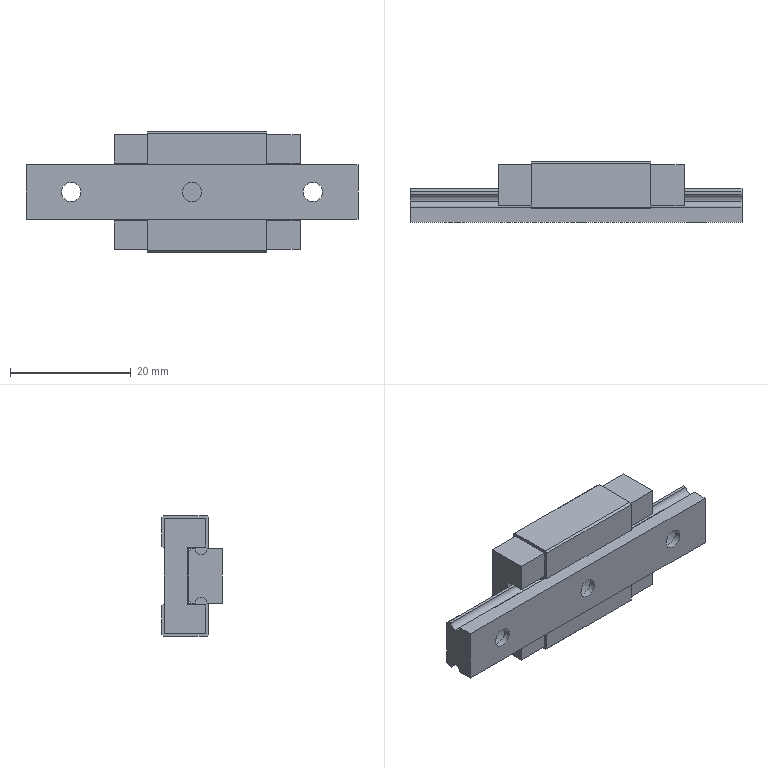Part | NX | 1 solid | 88 faces | box 55 x 10 x 20 mm | volume 5573 mm3 | plane 54 | cylinder 26 | cone 8 | commonest cylinder face diameters 2.5 x8 2 x6 3.2 x6 6.4 x6